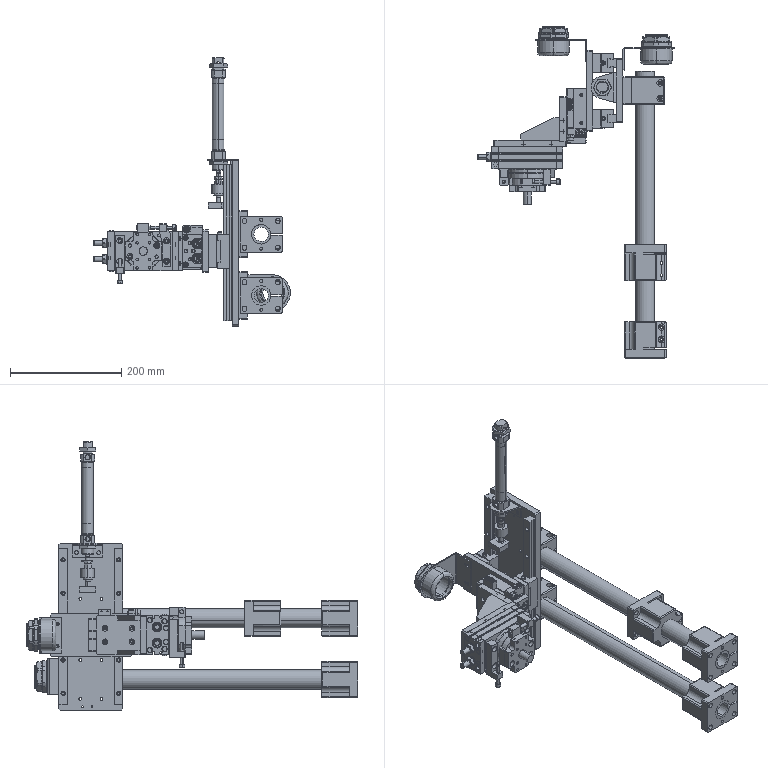Part | SolidWorks | features 3DProfileFeature 1 | 46 solids | 2645 faces | box 353.5 x 596.5 x 482 mm | volume 3186701 mm3 | cylinder 1102 | plane 1085 | cone 398 | spline 38 | torus 22 | commonest cylinder face diameters 4 x108 9 x65 5 x57 4.5 x56 4.917 x54 8 x44